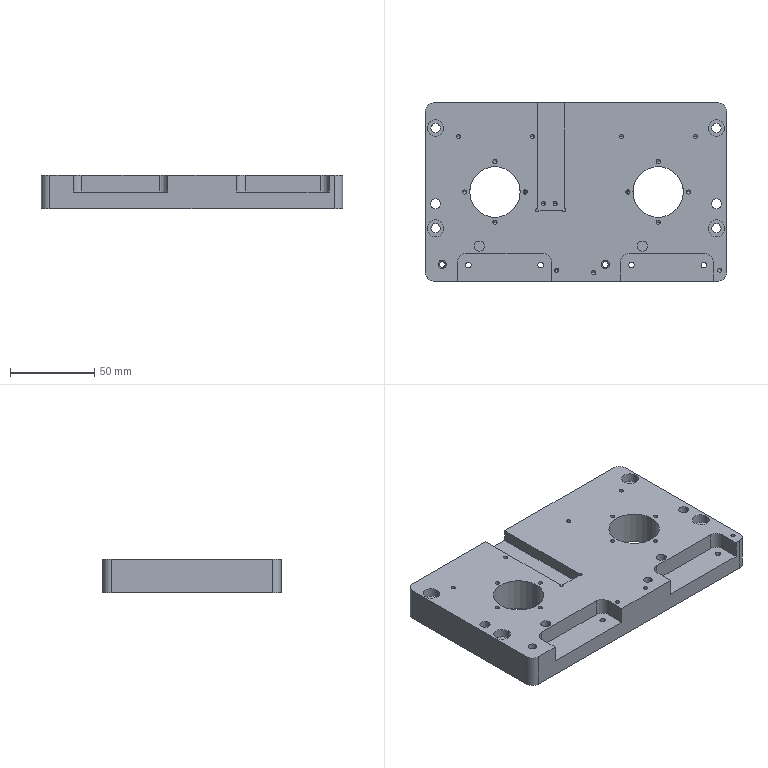Part | STEP file | 06-01-03 rotary base plate | 1 solid | 155 faces | box 179 x 106 x 20 mm | volume 319084 mm3 | cylinder 93 | cone 34 | plane 28 | commonest cylinder face diameters 2.5 x34 10 x16 3.3 x8 5.5 x8 6 x8 3.4 x4